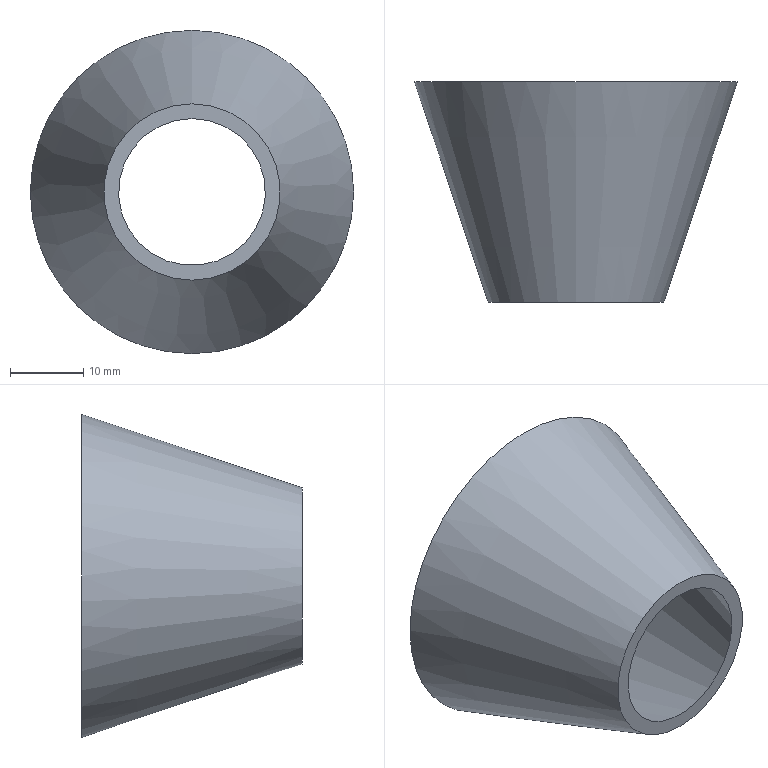Part | NX | features DATUM_CSYS 2, SKETCH 1, SWP104 1 | 1 solid | 4 faces | box 44 x 30 x 44 mm | volume 6032 mm3 | plane 2 | cone 2
STEP:
#1=CARTESIAN_POINT('',(0.,-30.,12.));
#2=VERTEX_POINT('',#1);
#3=CARTESIAN_POINT('',(0.,-30.,0.));
#4=DIRECTION('',(0.,1.,0.));
#5=DIRECTION('',(0.,0.,1.));
#6=AXIS2_PLACEMENT_3D('',#3,#4,#5);
#7=CIRCLE('',#6,12.);
#8=EDGE_CURVE('',#2,#2,#7,.T.);
#9=ORIENTED_EDGE('',*,*,#8,.F.);
#10=EDGE_LOOP('',(#9));
#11=FACE_BOUND('',#10,.T.);
#12=CARTESIAN_POINT('',(0.,-30.,10.));
#13=VERTEX_POINT('',#12);
#14=CARTESIAN_POINT('',(0.,-30.,0.));
#15=DIRECTION('',(0.,1.,0.));
#16=DIRECTION('',(0.,0.,1.));
#17=AXIS2_PLACEMENT_3D('',#14,#15,#16);
#18=CIRCLE('',#17,10.);
#19=EDGE_CURVE('',#13,#13,#18,.T.);
#20=ORIENTED_EDGE('',*,*,#19,.T.);
#21=EDGE_LOOP('',(#20));
#22=FACE_BOUND('',#21,.T.);
#23=CARTESIAN_POINT('',(10.,-30.,0.));
#24=DIRECTION('',(0.,1.,0.));
#25=DIRECTION('',(0.,0.,1.));
#26=AXIS2_PLACEMENT_3D('',#23,#24,#25);
#27=PLANE('',#26);
#28=ADVANCED_FACE('',(#11,#22),#27,.F.);
#29=CARTESIAN_POINT('',(0.,0.,22.));
#30=VERTEX_POINT('',#29);
#31=CARTESIAN_POINT('',(0.,0.,0.));
#32=DIRECTION('',(0.,1.,0.));
#33=DIRECTION('',(0.,0.,1.));
#34=AXIS2_PLACEMENT_3D('',#31,#32,#33);
#35=CIRCLE('',#34,22.);
#36=EDGE_CURVE('',#30,#30,#35,.T.);
#37=ORIENTED_EDGE('',*,*,#36,.F.);
#38=EDGE_LOOP('',(#37));
#39=FACE_BOUND('',#38,.T.);
#40=ORIENTED_EDGE('',*,*,#8,.T.);
#41=EDGE_LOOP('',(#40));
#42=FACE_BOUND('',#41,.T.);
#43=CARTESIAN_POINT('',(0.,-30.,0.));
#44=DIRECTION('',(0.,1.,0.));
#45=DIRECTION('',(0.,0.,1.));
#46=AXIS2_PLACEMENT_3D('',#43,#44,#45);
#47=CONICAL_SURFACE('',#46,12.,0.3218);
#48=ADVANCED_FACE('',(#39,#42),#47,.T.);
#49=CARTESIAN_POINT('',(0.,0.,20.));
#50=VERTEX_POINT('',#49);
#51=CARTESIAN_POINT('',(0.,0.,0.));
#52=DIRECTION('',(0.,1.,0.));
#53=DIRECTION('',(0.,0.,1.));
#54=AXIS2_PLACEMENT_3D('',#51,#52,#53);
#55=CIRCLE('',#54,20.);
#56=EDGE_CURVE('',#50,#50,#55,.T.);
#57=ORIENTED_EDGE('',*,*,#56,.F.);
#58=EDGE_LOOP('',(#57));
#59=FACE_BOUND('',#58,.T.);
#60=ORIENTED_EDGE('',*,*,#36,.T.);
#61=EDGE_LOOP('',(#60));
#62=FACE_BOUND('',#61,.T.);
#63=CARTESIAN_POINT('',(22.,0.,0.));
#64=DIRECTION('',(0.,-1.,0.));
#65=DIRECTION('',(0.,0.,-1.));
#66=AXIS2_PLACEMENT_3D('',#63,#64,#65);
#67=PLANE('',#66);
#68=ADVANCED_FACE('',(#59,#62),#67,.F.);
#69=ORIENTED_EDGE('',*,*,#19,.F.);
#70=EDGE_LOOP('',(#69));
#71=FACE_BOUND('',#70,.T.);
#72=ORIENTED_EDGE('',*,*,#56,.T.);
#73=EDGE_LOOP('',(#72));
#74=FACE_BOUND('',#73,.T.);
#75=CARTESIAN_POINT('',(0.,0.,0.));
#76=DIRECTION('',(0.,1.,0.));
#77=DIRECTION('',(0.,0.,1.));
#78=AXIS2_PLACEMENT_3D('',#75,#76,#77);
#79=CONICAL_SURFACE('',#78,20.,0.3218);
#80=ADVANCED_FACE('',(#71,#74),#79,.F.);
#81=CLOSED_SHELL('',(#28,#48,#68,#80));
#82=MANIFOLD_SOLID_BREP('',#81);
#83=(LENGTH_UNIT()NAMED_UNIT(*)SI_UNIT(.MILLI.,.METRE.));
#84=UNCERTAINTY_MEASURE_WITH_UNIT(LENGTH_MEASURE(0.00001),#83,'','');
#85=(NAMED_UNIT(*)PLANE_ANGLE_UNIT()SI_UNIT($,.RADIAN.));
#86=(NAMED_UNIT(*)SI_UNIT($,.STERADIAN.)SOLID_ANGLE_UNIT());
#87=(GEOMETRIC_REPRESENTATION_CONTEXT(3)GLOBAL_UNCERTAINTY_ASSIGNED_CONTEXT((#84))GLOBAL_UNIT_ASSIGNED_CONTEXT((#83,#85,#86))REPRESENTATION_CONTEXT('',''));
#88=ADVANCED_BREP_SHAPE_REPRESENTATION('',(#82),#87);